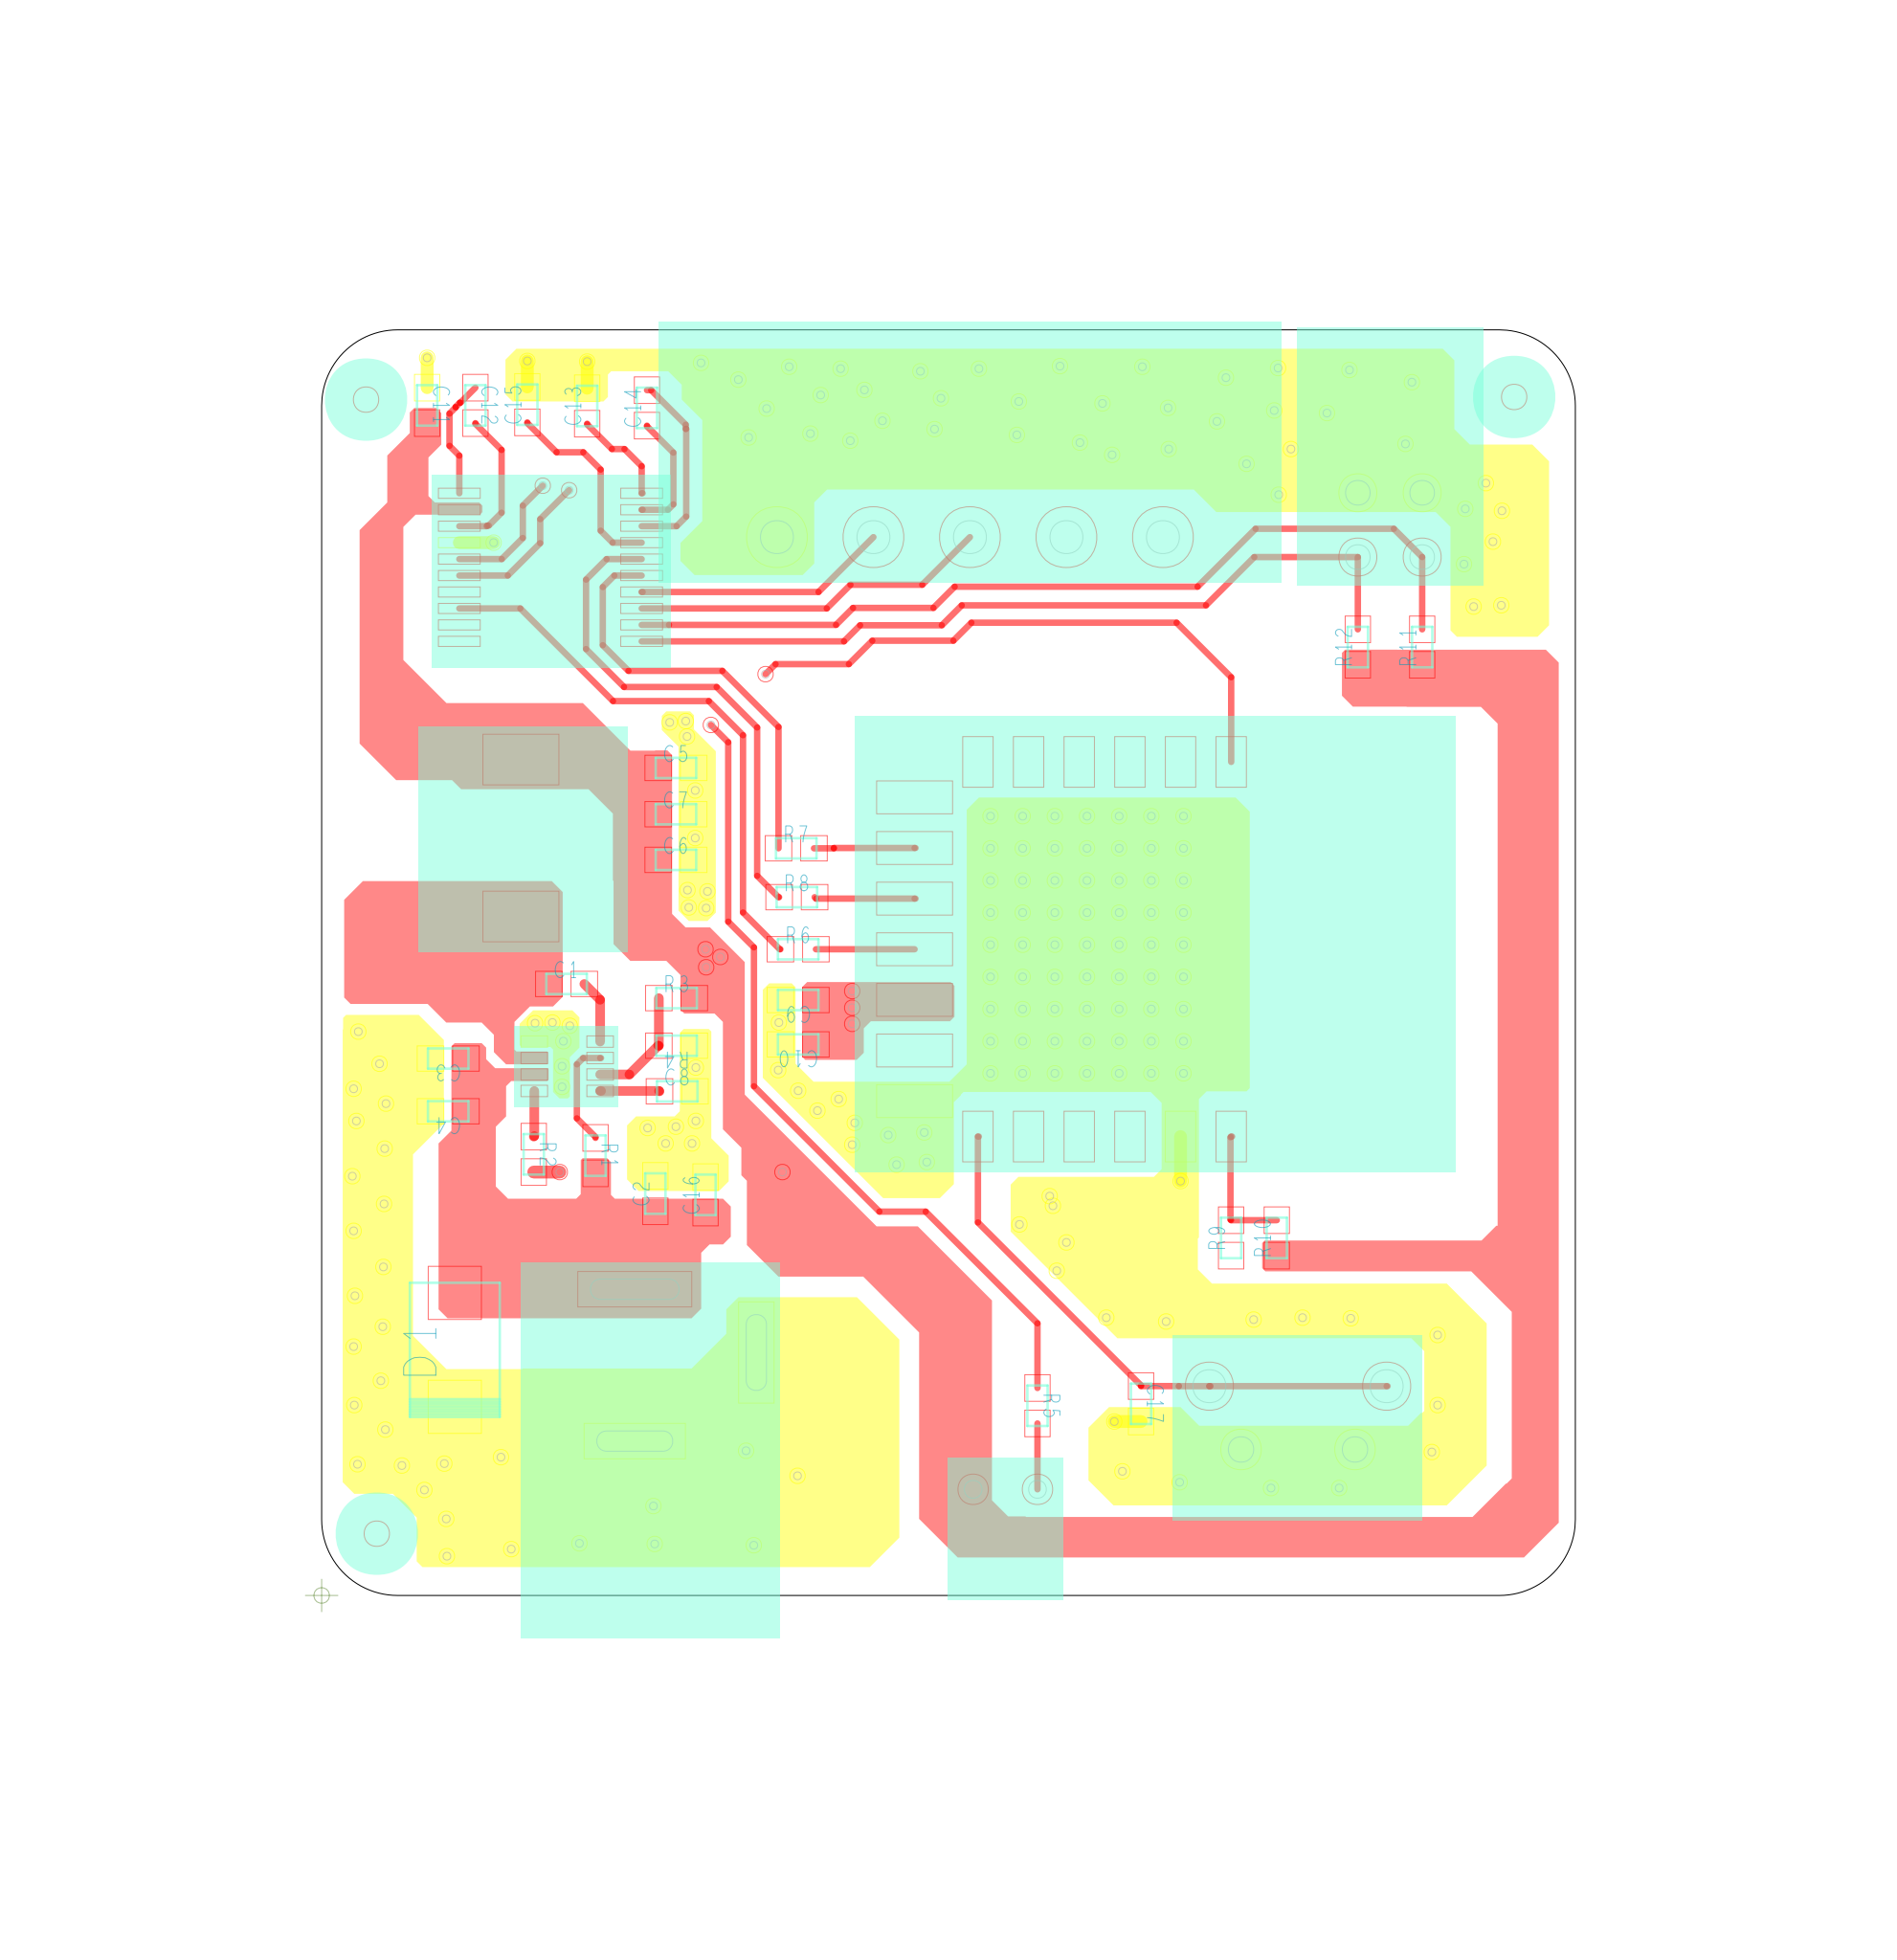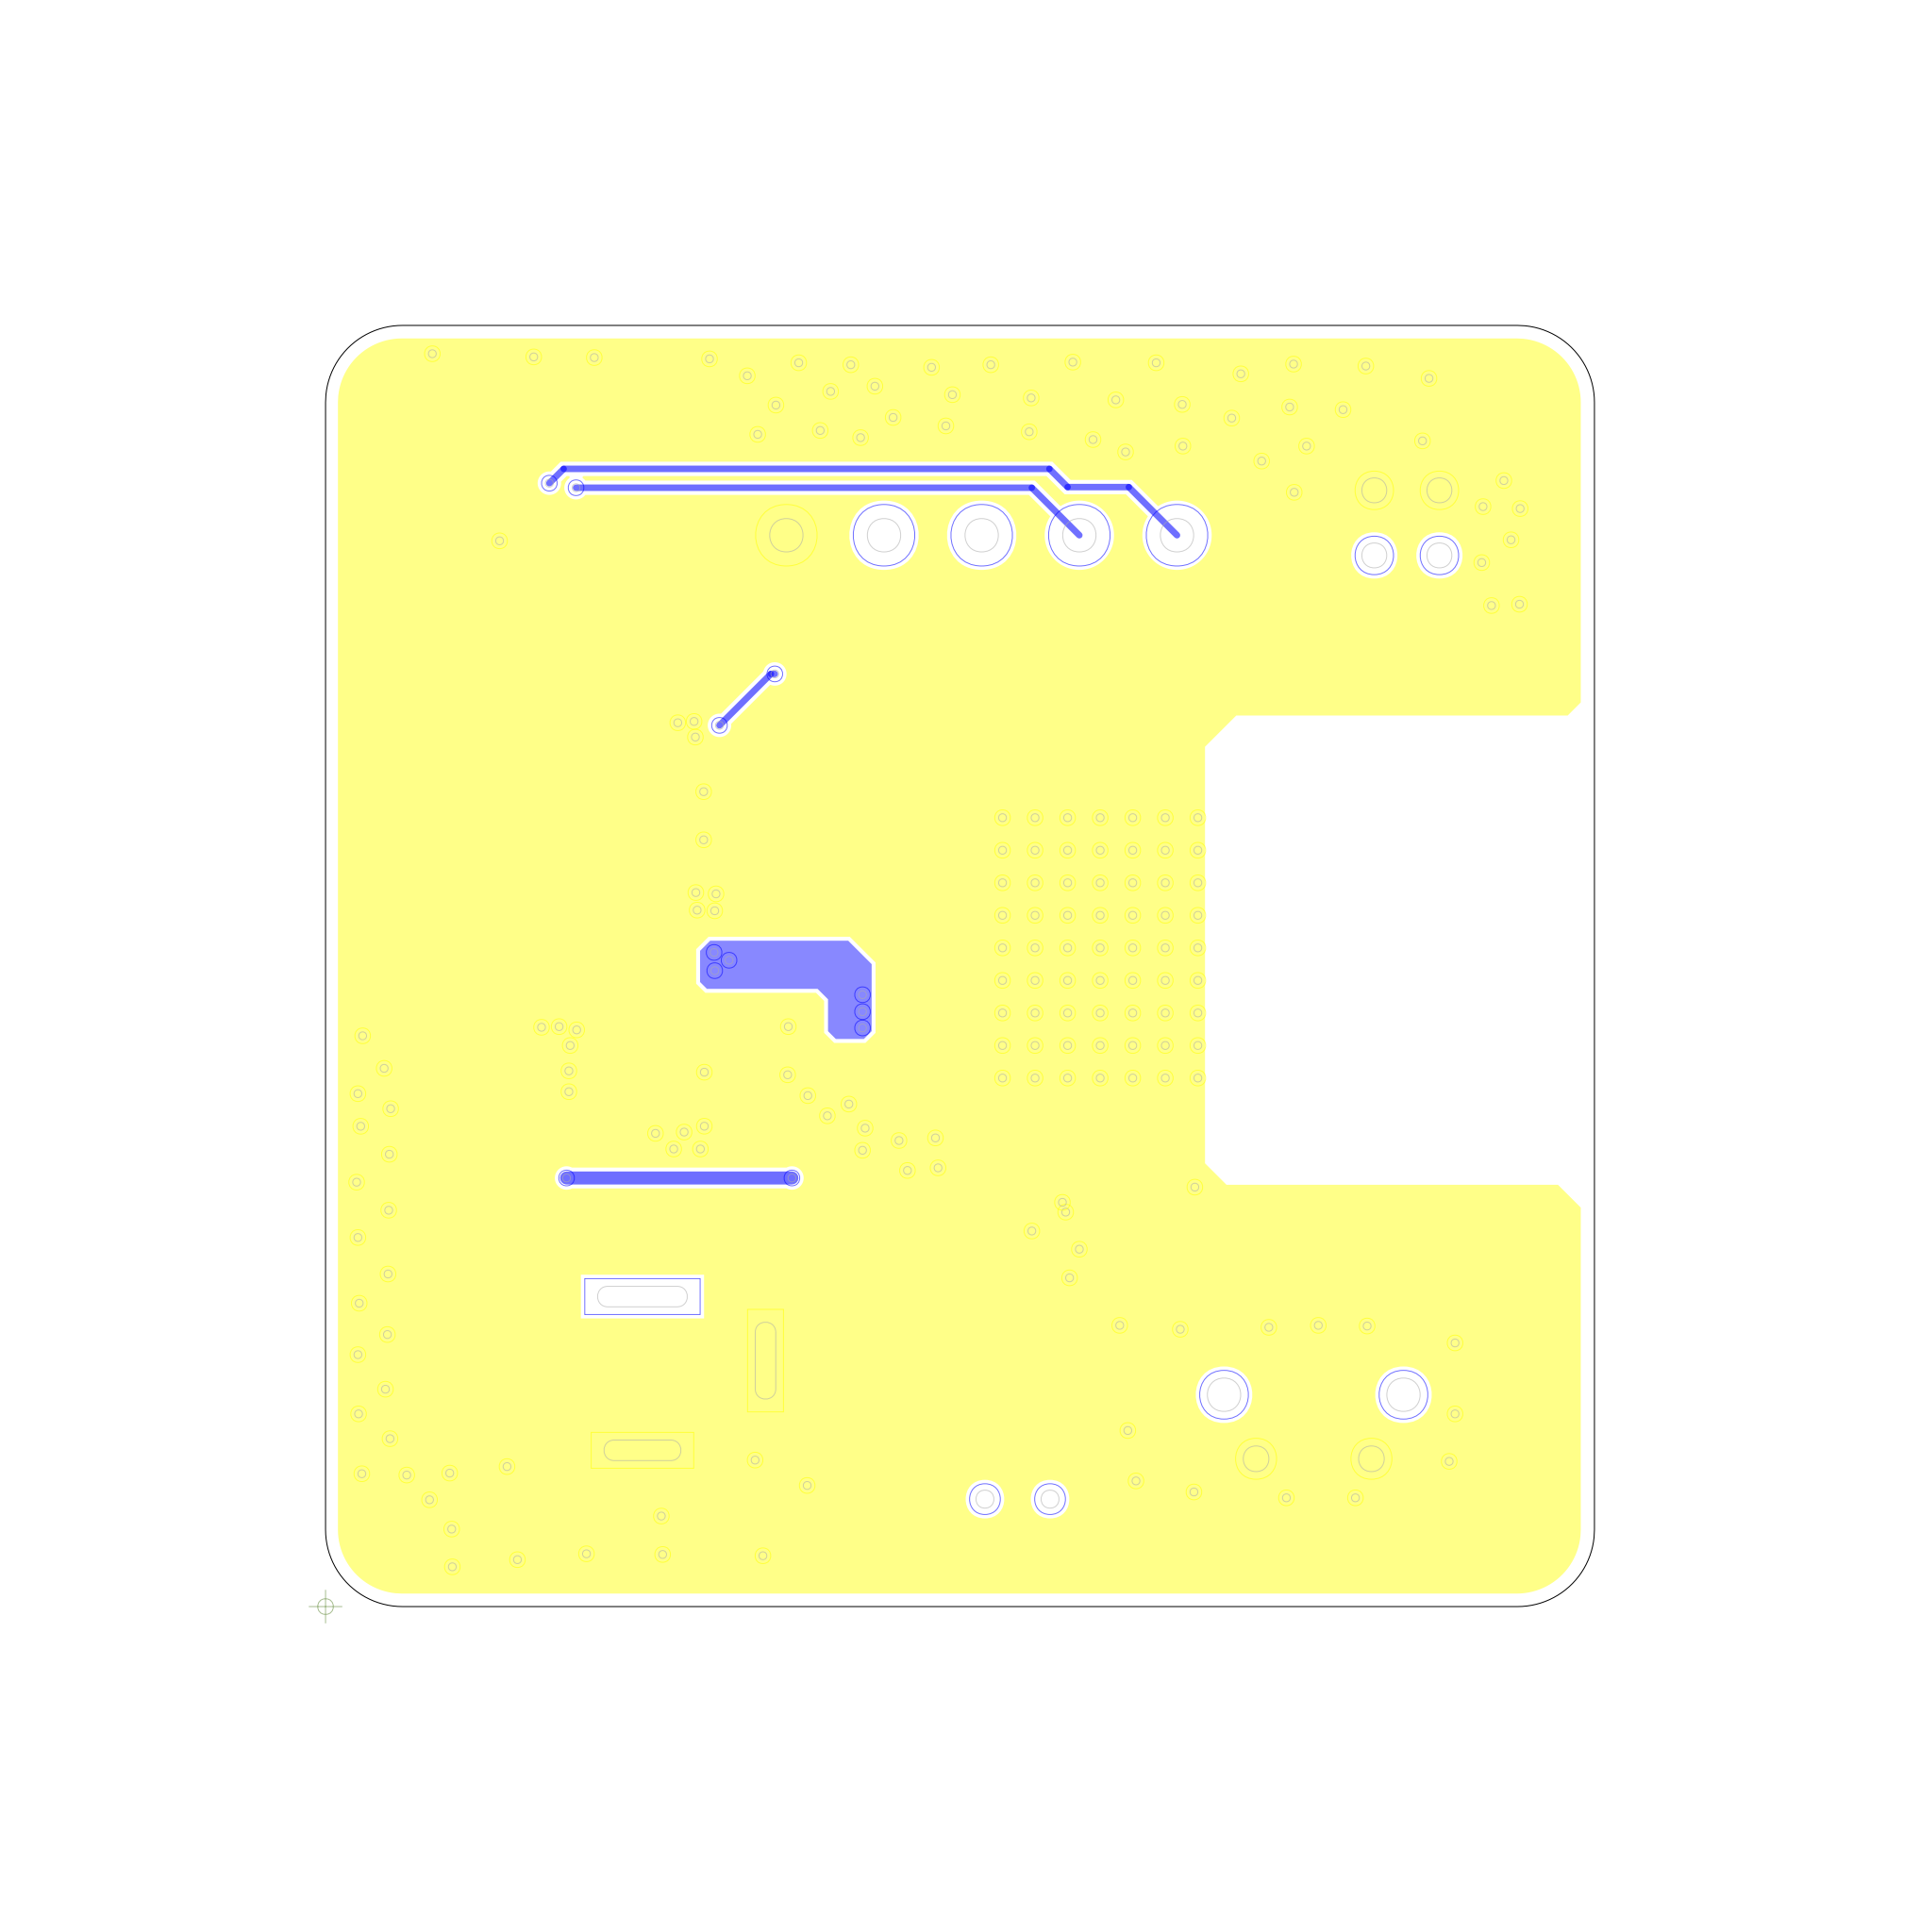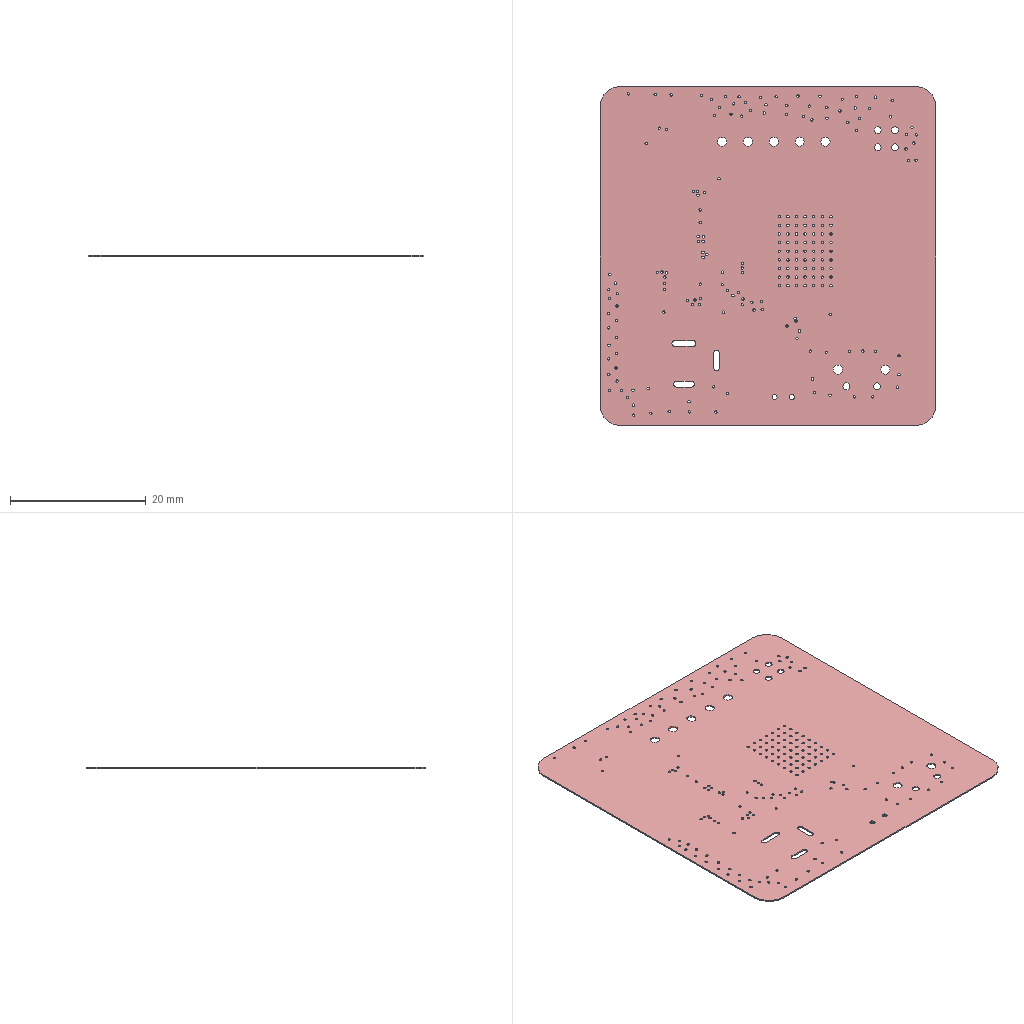Circuit board layout | Cadence Allegro | box 49.5 x 50 x 0.2 mm
Layer stack:
# Cadence Allegro layer stack of  (unit mm; from the constraint file cross-section; dielectric type: 0 not recorded (Allegro does not mark core vs prepreg), 3 surface material)
index,name,kind,layer,copper_thickness_mm,dielectric_type,dielectric_thickness_mm,dielectric_material,dielectric_constant
0,Top Surface,other,,,,,,
1,TOP,copper,TOP,0.0305,,,,
2,Dielectric1,dielectric,,,0,0.2032,FR-4,4.5
3,BOTTOM,copper,BOTTOM,0.0305,,,,
4,Bottom Surface,other,,,,,,
# drill layer pairs: low layer,high layer
drill_pair,TOP,BOTTOM
Part placement:
REFDES,COMP_VALUE,SYM_NAME,SYM_X,SYM_Y,SYM_ROTATE,SYM_MIRROR
C1,100nF/25V,C0603,380.728,951.102,0.000,NO
C2,100nF/25V,C0603,518.728,625.102,90.000,NO
C3,10uF/25V,C0603,196.728,835.102,180.000,NO
C4,10uF/25V,C0603,196.728,753.102,180.000,NO
C5,22uF/10V,C0603,550.728,1287.102,0.000,NO
C6,22uF/10V,C0603,550.728,1144.102,0.000,NO
C7,22uF/10V,C0603,550.728,1215.102,0.000,NO
C8,8200pF/10V,C0603,552.728,784.102,0.000,NO
C9,4.7uF,C0603,740.728,926.102,180.000,NO
C10,100nF,C0603,740.728,857.102,180.000,NO
C11,100nF/25V,C0603,164.000,1851.000,270.000,NO
C12,100nF/25V,C0603,239.000,1851.000,270.000,NO
C13,100nF/25V,C0603,412.728,1850.102,90.000,NO
C14,100nF/25V,C0603,505.728,1847.102,90.000,NO
C15,100nF/25V,C0603,319.728,1852.102,90.000,NO
C16,10uF/25V,C0603,596.728,623.102,90.000,NO
C17,100nF,C0603,1273.728,298.102,270.000,NO
D1,1SMB18CAT3G,SMB,207.000,382.000,90.000,NO
J1,CON6,JK2EDGRC-381-5_1,1007.728,1646.102,180.000,NO
J16,DC-005,DC-005,486.728,240.102,90.000,NO
L1,MS73-2R2NT,SMD7X7,309.728,1178.102,180.000,NO
LED1,LED_GREEN,LEDC1608X60N,1062.728,165.102,0.000,NO
R1,510K,R0603,425.728,684.102,270.000,NO
R2,100K,R0603,329.728,686.102,270.000,NO
R3,33.2K,R0603,551.728,929.102,0.000,NO
R4,10K,R0603,551.728,855.102,180.000,NO
R5,1K,R0603,1112.728,295.102,270.000,NO
R6,10R,R0603,740.728,1005.102,0.000,NO
R7,10R,R0603,737.728,1162.102,0.000,NO
R8,10R,R0603,738.728,1086.102,0.000,NO
R9,NC,R0603,1413.728,556.102,90.000,NO
R10,10K,R0603,1484.728,556.102,90.000,NO
R11,4K7,R0603,1710.728,1475.102,90.000,NO
R12,4K7,R0603,1610.728,1475.102,90.000,NO
SW1,SW DIP-2,DA-02,1660.728,1715.102,180.000,NO
SW2,SW PUSHBUTTON-SPST-2,DIP-4,1517.728,227.102,0.000,NO
U1,TPS562219ADDFT,SOT-8,381.728,823.102,0.000,NO
U2,DS-REX3B,DS-REX3B,921.728,1005.102,0.000,NO
U3,XR3160,TSSOP-20_1,355.728,1599.102,0.000,NO
Pad and via stacks:
# Allegro (Cadence) via spans and padstacks; design units: ("mils" 3 1000)
# via spans: padstack,start_layer,end_layer,net_example,count
VIA12_24,ETCH/TOP,ETCH/BOTTOM,GND,202
# Allegro padstack definitions: name,start_layer,end_layer,drill,plating,holeType,type
R180_160,"ETCH/TOP","ETCH/TOP",0.0,"PLATED","none","smd"
RE118_11X98_43,"ETCH/TOP","ETCH/TOP",0.0,"NON_PLATED","none","smd"
R105_100,"ETCH/TOP","ETCH/TOP",0.0,"PLATED","none","smd"
R170_135,"ETCH/TOP","ETCH/TOP",0.0,"PLATED","none","smd"
R145_120,"ETCH/TOP","ETCH/TOP",0.0,"PLATED","none","smd"
RE350X100,"ETCH/TOP","ETCH/TOP",0.0,"PLATED","none","smd"
RE55X40,"ETCH/TOP","ETCH/TOP",0.0,"NON_PLATED","none","smd"
R225_160,"ETCH/TOP","ETCH/TOP",0.0,"PLATED","none","smd"
S210,"ETCH/TOP","ETCH/TOP",0.0,"PLATED","none","smd"
RE90X95,"ETCH/TOP","ETCH/TOP",0.0,"NON_PLATED","none","smd"
SMD_R787X1181P0S40,"ETCH/TOP","ETCH/TOP",0.0,"PLATED","none","smd"
SMD_R98X472P0S40,"ETCH/TOP","ETCH/TOP",0.0,"PLATED","none","smd"
SMD_R472X709P0S40,"ETCH/TOP","ETCH/TOP",0.0,"PLATED","none","smd"
SMD_R276X709P0S40,"ETCH/TOP","ETCH/TOP",0.0,"PLATED","none","smd"
SMD_R591X1102P0S40,"ETCH/TOP","ETCH/TOP",0.0,"PLATED","none","smd"
SMD_R433X709P0S40,"ETCH/TOP","ETCH/TOP",0.0,"PLATED","none","smd"
SMD_R984X787P0S40,"ETCH/TOP","ETCH/TOP",0.0,"PLATED","none","smd"
SMD_R236X787P0S40,"ETCH/TOP","ETCH/TOP",0.0,"PLATED","none","smd"
RE200X125,"ETCH/TOP","ETCH/TOP",0.0,"PLATED","none","smd"
RE75X40,"ETCH/TOP","ETCH/TOP",0.0,"NON_PLATED","none","smd"
SQ120,"ETCH/TOP","ETCH/TOP",0.0,"PLATED","none","smd"
RE620X580,"ETCH/TOP","ETCH/TOP",0.0,"NON_PLATED","none","smd"
RE300X160,"ETCH/TOP","ETCH/TOP",0.0,"NON_PLATED","none","smd"
R105_45,"ETCH/TOP","ETCH/TOP",0.0,"PLATED","none","smd"
RE65X180,"ETCH/TOP","ETCH/TOP",0.0,"PLATED","none","smd"
SMD_R100X650P0S40,"ETCH/TOP","ETCH/TOP",0.0,"PLATED","none","smd"
RE150X80,"ETCH/TOP","ETCH/TOP",0.0,"NON_PLATED","none","smd"
SMD_R512X413P0S40,"ETCH/TOP","ETCH/TOP",0.0,"PLATED","none","smd"
RE60X24,"ETCH/TOP","ETCH/TOP",0.0,"NON_PLATED","none","smd"
RE43_31X19_68,"ETCH/TOP","ETCH/TOP",0.0,"PLATED","none","smd"
RE134X170,"ETCH/TOP","ETCH/TOP",0.0,"PLATED","none","smd"
R110_60,"ETCH/TOP","ETCH/TOP",0.0,"PLATED","none","smd"
RE100X150,"ETCH/TOP","ETCH/TOP",0.0,"PLATED","none","smd"
RE330X150,"ETCH/TOP","ETCH/TOP",0.0,"PLATED","none","smd"
RE39_37X11_81,"ETCH/TOP","ETCH/TOP",0.0,"NON_PLATED","none","smd"
RE11_81X39_37,"ETCH/TOP","ETCH/TOP",0.0,"NON_PLATED","none","smd"
SQ124,"ETCH/TOP","ETCH/TOP",0.0,"NON_PLATED","none","smd"
SQ20,"ETCH/TOP","ETCH/TOP",0.0,"NON_PLATED","none","smd"
R155_60,"ETCH/TOP","ETCH/TOP",0.0,"PLATED","none","smd"
SMD_R118X315P0S40,"ETCH/TOP","ETCH/TOP",0.0,"PLATED","none","smd"
R27X39,"ETCH/TOP","ETCH/TOP",0.0,"PLATED","none","smd"
SMD_R98X315P0S40,"ETCH/TOP","ETCH/TOP",0.0,"PLATED","none","smd"
SMD_S984P0S40,"ETCH/TOP","ETCH/TOP",0.0,"PLATED","none","smd"
SMD_R591X295P0S40,"ETCH/TOP","ETCH/TOP",0.0,"PLATED","none","smd"
SMD_R295X591P0S40,"ETCH/TOP","ETCH/TOP",0.0,"PLATED","none","smd"
B160_60,"ETCH/TOP","ETCH/TOP",0.0,"PLATED","none","smd"
R18X20,"ETCH/TOP","ETCH/TOP",0.0,"NON_PLATED","none","smd"
Y3,"ETCH/TOP","ETCH/TOP",0.0,"PLATED","none","smd"
R1651X3,"ETCH/TOP","ETCH/TOP",0.0,"PLATED","none","smd"
R25X14,"ETCH/TOP","ETCH/TOP",0.0,"PLATED","none","smd"
R17X13,"ETCH/TOP","ETCH/TOP",0.0,"PLATED","none","smd"
R3X2,"ETCH/TOP","ETCH/TOP",0.0,"PLATED","none","smd"
VIA30D16,"ETCH/TOP","ETCH/BOTTOM",16.0,"PLATED","circle_drill","through"
PTH_C472D276S40,"ETCH/TOP","ETCH/BOTTOM",27.559,"PLATED","circle_drill","through"
PTH_S472D276S40,"ETCH/TOP","ETCH/BOTTOM",27.559,"PLATED","circle_drill","through"
C43_31D43_31,"ETCH/TOP","ETCH/BOTTOM",43.311,"PLATED","circle_drill","through"
S220H120T220_240_40,"ETCH/TOP","ETCH/BOTTOM",47.244,"PLATED","circle_drill","through"
C220H120T220_240_40,"ETCH/TOP","ETCH/BOTTOM",47.244,"PLATED","circle_drill","through"
S160H105T155_190_40,"ETCH/TOP","ETCH/BOTTOM",41.339,"PLATED","circle_drill","through"
C160H105T155_190_40,"ETCH/TOP","ETCH/BOTTOM",41.339,"PLATED","circle_drill","through"
PTH_O1800X800SLOT500X1100S40,"ETCH/TOP","ETCH/BOTTOM",50.0,"PLATED","oval slot","through"
PTH_O800X1800SLOT500X1200S40,"ETCH/TOP","ETCH/BOTTOM",50.0,"PLATED","oval slot","through"
PTH_O800X1800SLOT500X1100S40,"ETCH/TOP","ETCH/BOTTOM",50.0,"PLATED","oval slot","through"
PTH_S630D362S40,"ETCH/TOP","ETCH/BOTTOM",36.22,"PLATED","circle_drill","through"
PTH_C630D362S40,"ETCH/TOP","ETCH/BOTTOM",36.22,"PLATED","circle_drill","through"
PTH_C1496D906S40,"ETCH/TOP","ETCH/BOTTOM",90.551,"PLATED","circle_drill","through"
S140H80,"ETCH/TOP","ETCH/BOTTOM",31.496,"PLATED","circle_drill","through"
C140H80,"ETCH/TOP","ETCH/BOTTOM",31.496,"PLATED","circle_drill","through"
S140H90T140_170_40,"ETCH/TOP","ETCH/BOTTOM",35.433,"PLATED","circle_drill","through"
C140H90T140_170_40,"ETCH/TOP","ETCH/BOTTOM",35.433,"PLATED","circle_drill","through"
C355H235T285_330_50,"ETCH/TOP","ETCH/BOTTOM",92.52,"PLATED","circle_drill","through"
PTH_C591D402S40,"ETCH/TOP","ETCH/BOTTOM",40.161,"PLATED","circle_drill","through"
PTH_C600D350S40,"ETCH/TOP","ETCH/BOTTOM",35.0,"PLATED","circle_drill","through"
PTH_C866D650S40,"ETCH/TOP","ETCH/BOTTOM",64.961,"PLATED","circle_drill","through"
PTH_S600D350S40,"ETCH/TOP","ETCH/BOTTOM",35.0,"PLATED","circle_drill","through"
C100H60,"ETCH/TOP","ETCH/BOTTOM",23.622,"PLATED","circle_drill","through"
RE100H60,"ETCH/TOP","ETCH/BOTTOM",23.622,"PLATED","circle_drill","through"
H70,"ETCH/TOP","ETCH/BOTTOM",27.559,"PLATED","circle_drill","through"
PTH_C600D300S40,"ETCH/TOP","ETCH/BOTTOM",30.0,"PLATED","circle_drill","through"
C177_17D137_80,"ETCH/TOP","ETCH/BOTTOM",137.799,"PLATED","circle_drill","through"
PTH_O1024X709SLOT394X630S40,"ETCH/TOP","ETCH/BOTTOM",39.37,"PLATED","oval slot","through"
VIA12_24,"ETCH/TOP","ETCH/BOTTOM",12.0,"PLATED","circle_drill","through"
Y300,"ETCH/TOP","ETCH/BOTTOM",118.11,"NON_PLATED","circle_drill","through"
C83D53,"ETCH/TOP","ETCH/BOTTOM",53.0,"PLATED","circle_drill","through"
Y97,"ETCH/TOP","ETCH/BOTTOM",38.189,"PLATED","circle_drill","through"
Y700,"ETCH/TOP","ETCH/BOTTOM",27.559,"PLATED","circle_drill","through"
Y200,"ETCH/TOP","ETCH/BOTTOM",51.181,"PLATED","circle_drill","through"
Y170,"ETCH/TOP","ETCH/BOTTOM",39.37,"PLATED","circle_drill","through"
R350X80,"ETCH/TOP","ETCH/BOTTOM",31.496,"PLATED","oval slot","through"
R300X80,"ETCH/TOP","ETCH/BOTTOM",31.496,"PLATED","oval slot","through"
Y24,"ETCH/TOP","ETCH/BOTTOM",51.181,"PLATED","circle_drill","through"
Design rules, without the lines most boards share, first 13 of 24 lines:
# Cadence Allegro design rules of  (from the Constraint Manager export constraints.dcfx, design unit mil; typed fields in mm)
# columns: name | kind | enabled | priority | scope1 | scope2 | descriptor | typed fields (field=value)
# Allegro precedence (priority 1 wins): 1 Region class-to-class, 2 Region class, 3 Region, 4 class-to-class, 5 DiffPair/Bus/NetGroup override, 6 NetClass, 7 constraint set (CSet) default
# per-layer values are written LAYER=value in the descriptor and LAYER:mm in the typed field; a maximum of 0 means no limit set
# --- net classes (and buses / net groups) ---
# (no net classes defined: every net uses the default constraint sets)
# --- track widths, neck and differential-pair gap (physical constraint sets) ---
DEFAULT | PhysicalCSet | enabled | 7 | Design default | All | Physical Constraint (Min Line Width=10mil) (Max Line Width=100mil) (Min Neck Width=6mil) (Max Neck Length=6mil) (DiffPair Primary Gap=6mil) (DiffPair Neck Gap=6mil) (DiffPair Min Space=6mil) (DiffPair Coupled +Tol=6mil) (DiffPair Coupled -Tol=6mil) (Min BB Via Stagger=6mil) (Max BB Via Stagger=6mil) (T-junctions=ANYWHERE) (Pad-pad direct connect=ALL_ALLOWED) (Allowed vias=VIA12_24) | min_line_width=0.254 min_neck_width=0.1524 min_bvia_stagger=0.1524 max_bvia_stagger=0.1524 ts_allowed=ANYWHERE diffp_primary_gap=0.1524 diffp_neck_gap=0.1524 max_line_width=2.54 maximum_neck_length=0.1524 pad_pad_direct_connect=ALL_ALLOWED allow_on_etch_subclass=TRUE diffp_coupled_plus=0.1524 diffp_coupled_minus=0.1524 diffp_min_space=0.1524 vias=VIA12_24
# --- clearances: line / pad / via / shape / hole (spacing constraint sets) ---
DEFAULT | SpacingCSet | enabled | 7 | Design default | All | Clearance Constraint (Line-Line=6mil) (Line-SMD Pad=6mil) (Line-Thru Pin=6mil) (Line-Via=6mil) (Line-Shape=6mil) (SMD Pad-SMD Pad=7mil) (Thru Pin-Thru Pin=7mil) (Thru Pin-SMD Pad=7mil) (SMD Pad-Via=6mil) (Thru Pin-Via=6mil) (Via-Via=6mil) (Shape-SMD Pad=6mil) (Shape-Thru Pin=6mil) (Shape-Via=6mil) (Shape-Shape=6mil) (Hole-Hole=8mil) (Hole-Line=6mil) (Hole-Shape=8mil) (BB Via-BB Via=6mil) (uVia-uVia=5mil) | thrupin_to_thrupin_spacing=0.1778 thrupin_to_smdpin_spacing=0.1778 thrupin_to_thruvia_spacing=0.1524 line_to_thrupin_spacing=0.1524 thrupin_to_shape_spacing=0.1524 smdpin_to_smdpin_spacing=0.1778 smdpin_to_thruvia_spacing=0.1524 line_to_smdpin_spacing=0.1524 shape_to_smdpin_spacing=0.1524 thruvia_to_thruvia_spacing=0.1524 line_to_thruvia_spacing=0.1524 shape_to_thruvia_spacing=0.1524 line_to_line_spacing=0.1524 line_to_shape_spacing=0.1524 shape_to_shape_spacing=0.1524 bbv_to_bbv_spacing=0.1524 bbv_to_thrupin_spacing=0.1524 bbv_to_smdpin_spacing=0.1524 bbv_to_thruvia_spacing=0.1524 bbv_to_line_spacing=0.1524 bbv_to_shape_spacing=0.1524 bbv_to_testpin_spacing=0.1524 bbv_to_testvia_spacing=0.1524 testpin_to_testpin_spacing=0.1778 testpin_to_thrupin_spacing=0.1778 smdpin_to_testpin_spacing=0.1778 testpin_to_thruvia_spacing=0.1524 testpin_to_testvia_spacing=0.1524 line_to_testpin_spacing=0.1524 shape_to_testpin_spacing=0.1524 testvia_to_testvia_spacing=0.127 testvia_to_thrupin_spacing=0.1524 smdpin_to_testvia_spacing=0.1524 testvia_to_thruvia_spacing=0.1524 line_to_testvia_spacing=0.1524 shape_to_testvia_spacing=0.1524 bondpad_to_bondpad_spacing=0.127 thrupin_to_bondpad_spacing=0.1524 smdpin_to_bondpad_spacing=0.1524 bondpad_to_thruvia_spacing=0.1524 bondpad_to_line_spacing=0.1524 bondpad_to_shape_spacing=0.1524 bondpad_to_bbv_spacing=0.1524 bondpad_to_testpin_spacing=0.1524 bondpad_to_testvia_spacing=0.127 min_bvia_gap=0.127 hole_to_pin_spacing=0.2032 hole_to_via_spacing=0.2032 hole_to_line_spacing=0.1524 hole_to_shape_spacing=0.2032 hole_to_hole_spacing=0.2032 mvia_to_mvia_spacing=0.127 mvia_to_thrupin_spacing=0.127 mvia_to_smdpin_spacing=0.127 mvia_to_thruvia_spacing=0.127 mvia_to_bbv_spacing=0.127 mvia_to_line_spacing=0.127 mvia_to_shape_spacing=0.127 mvia_to_testpin_spacing=0.127 mvia_to_testvia_spacing=0.127 bondpad_to_mvia_spacing=0.127 bondpad_to_bondpad_diffp_spc=0.127
DEFAULT | SameNetSpacingCSet | enabled | 7 | Design default | All | Same-Net Clearance (Line-Line=5mil) (Line-SMD Pad=5mil) (Line-Thru Pin=5mil) (Line-Via=5mil) (Line-Shape=5mil) (SMD Pad-SMD Pad=5mil) (Thru Pin-Thru Pin=5mil) (Thru Pin-SMD Pad=5mil) (SMD Pad-Via=5mil) (Thru Pin-Via=5mil) (Via-Via=5mil) (Shape-SMD Pad=5mil) (Shape-Thru Pin=5mil) (Shape-Via=5mil) (Shape-Shape=5mil) (Hole-Hole=8mil) (Hole-Line=8mil) (Hole-Shape=8mil) (BB Via-BB Via=5mil) (uVia-uVia=5mil) | sn_thrupin_to_thrupin_spacing=0.127 sn_thrupin_to_smdpin_spacing=0.127 sn_thrupin_to_thruvia_spacing=0.127 sn_line_to_thrupin_spacing=0.127 sn_thrupin_to_shape_spacing=0.127 sn_smdpin_to_smdpin_spacing=0.127 sn_smdpin_to_thruvia_spacing=0.127 sn_line_to_smdpin_spacing=0.127 sn_shape_to_smdpin_spacing=0.127 sn_thruvia_to_thruvia_spacing=0.127 sn_line_to_thruvia_spacing=0.127 sn_shape_to_thruvia_spacing=0.127 sn_line_to_line_spacing=0.127 sn_line_to_shape_spacing=0.127 sn_shape_to_shape_spacing=0.127 sn_bbv_to_bbv_spacing=0.127 sn_bbv_to_thrupin_spacing=0.127 sn_bbv_to_smdpin_spacing=0.127 sn_bbv_to_thruvia_spacing=0.127 sn_bbv_to_line_spacing=0.127 sn_bbv_to_shape_spacing=0.127 sn_bbv_to_testpin_spacing=0.127 sn_bbv_to_testvia_spacing=0.127 sn_testpin_to_testpin_spacing=0.127 sn_testpin_to_thrupin_spacing=0.127 sn_smdpin_to_testpin_spacing=0.127 sn_testpin_to_thruvia_spacing=0.127 sn_testpin_to_testvia_spacing=0.127 sn_line_to_testpin_spacing=0.127 sn_shape_to_testpin_spacing=0.127 sn_testvia_to_testvia_spacing=0.127 sn_testvia_to_thrupin_spacing=0.127 sn_smdpin_to_testvia_spacing=0.127 sn_testvia_to_thruvia_spacing=0.127 sn_line_to_testvia_spacing=0.127 sn_shape_to_testvia_spacing=0.127 sn_bondpad_to_bondpad_spacing=0.127 sn_thrupin_to_bondpad_spacing=0.127 sn_smdpin_to_bondpad_spacing=0.127 sn_bondpad_to_thruvia_spacing=0.127 sn_bondpad_to_line_spacing=0.127 sn_bondpad_to_shape_spacing=0.127 sn_bondpad_to_bbv_spacing=0.127 sn_bondpad_to_testpin_spacing=0.127 sn_bondpad_to_testvia_spacing=0.127 same_net=TRUE sn_hole_to_pin_spacing=0.2032 sn_hole_to_via_spacing=0.2032 sn_hole_to_line_spacing=0.2032 sn_hole_to_shape_spacing=0.2032 sn_hole_to_hole_spacing=0.2032 sn_mvia_to_mvia_spacing=0.127 sn_mvia_to_thrupin_spacing=0.127 sn_mvia_to_smdpin_spacing=0.127 sn_mvia_to_thruvia_spacing=0.127 sn_mvia_to_bbv_spacing=0.127 sn_mvia_to_line_spacing=0.127 sn_mvia_to_shape_spacing=0.127 sn_mvia_to_testpin_spacing=0.127 sn_mvia_to_testvia_spacing=0.127 sn_bondpad_to_mvia_spacing=0.127
# --- differential pairs (0) ---
# (no differential pairs defined)